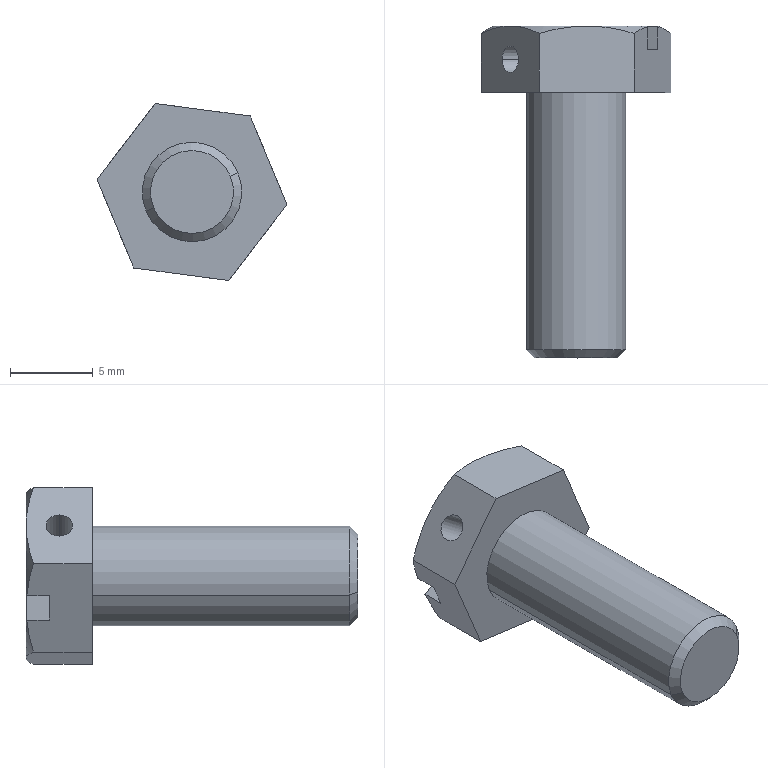Part | SolidWorks | features BaseBody 1 | 1 solid | 26 faces | box 11.449 x 20 x 10.666 mm | volume 753.247 mm3 | plane 14 | cone 8 | cylinder 4 | commonest cylinder face diameters 1.6 x2 6 x2
STEP:
#1=CARTESIAN_POINT('',(325.991,230.1,-29.958));
#2=VERTEX_POINT('',#1);
#3=CARTESIAN_POINT('',(330.609,230.1,-28.042));
#4=VERTEX_POINT('',#3);
#5=CARTESIAN_POINT('',(328.3,230.1,-29.));
#6=DIRECTION('',(0.,-1.,0.));
#7=DIRECTION('',(-0.9237,0.,-0.383));
#8=AXIS2_PLACEMENT_3D('',#5,#6,#7);
#9=CIRCLE('',#8,2.5);
#10=EDGE_CURVE('',#2,#4,#9,.T.);
#11=ORIENTED_EDGE('',*,*,#10,.F.);
#12=CARTESIAN_POINT('',(325.529,230.6,-30.149));
#13=VERTEX_POINT('',#12);
#14=CARTESIAN_POINT('',(325.529,230.6,-30.149));
#15=DIRECTION('',(-0.6532,0.7071,-0.2709));
#16=VECTOR('',#15,1000.);
#17=LINE('',#14,#16);
#18=EDGE_CURVE('',#2,#13,#17,.T.);
#19=ORIENTED_EDGE('',*,*,#18,.T.);
#20=CARTESIAN_POINT('',(331.071,230.6,-27.851));
#21=VERTEX_POINT('',#20);
#22=CARTESIAN_POINT('',(328.3,230.6,-29.));
#23=DIRECTION('',(0.,1.,0.));
#24=DIRECTION('',(-0.9237,0.,-0.383));
#25=AXIS2_PLACEMENT_3D('',#22,#23,#24);
#26=CIRCLE('',#25,3.);
#27=EDGE_CURVE('',#21,#13,#26,.T.);
#28=ORIENTED_EDGE('',*,*,#27,.F.);
#29=CARTESIAN_POINT('',(331.071,230.6,-27.851));
#30=DIRECTION('',(0.6532,0.7071,0.2709));
#31=VECTOR('',#30,1000.);
#32=LINE('',#29,#31);
#33=EDGE_CURVE('',#4,#21,#32,.T.);
#34=ORIENTED_EDGE('',*,*,#33,.F.);
#35=EDGE_LOOP('',(#11,#19,#28,#34));
#36=FACE_OUTER_BOUND('',#35,.T.);
#37=CARTESIAN_POINT('',(328.3,230.6,-29.));
#38=DIRECTION('',(0.,1.,0.));
#39=DIRECTION('',(0.9237,0.,0.383));
#40=AXIS2_PLACEMENT_3D('',#37,#38,#39);
#41=CONICAL_SURFACE('',#40,3.,0.7854);
#42=ADVANCED_FACE('',(#36),#41,.T.);
#43=CARTESIAN_POINT('',(332.755,248.1,-31.407));
#44=VERTEX_POINT('',#43);
#45=CARTESIAN_POINT('',(331.781,248.1,-32.677));
#46=VERTEX_POINT('',#45);
#47=CARTESIAN_POINT('',(332.268,248.1,-32.042));
#48=DIRECTION('',(0.7936,0.,-0.6084));
#49=DIRECTION('',(-0.6084,0.,-0.7936));
#50=AXIS2_PLACEMENT_3D('',#47,#48,#49);
#51=CIRCLE('',#50,0.8);
#52=EDGE_CURVE('',#44,#46,#51,.T.);
#53=ORIENTED_EDGE('',*,*,#52,.T.);
#54=CARTESIAN_POINT('',(323.845,248.1,-26.593));
#55=VERTEX_POINT('',#54);
#56=CARTESIAN_POINT('',(333.766,248.1,-34.199));
#57=DIRECTION('',(-0.7936,0.,0.6084));
#58=VECTOR('',#57,1000.);
#59=LINE('',#56,#58);
#60=EDGE_CURVE('',#46,#55,#59,.T.);
#61=ORIENTED_EDGE('',*,*,#60,.T.);
#62=CARTESIAN_POINT('',(324.819,248.1,-25.323));
#63=VERTEX_POINT('',#62);
#64=CARTESIAN_POINT('',(324.332,248.1,-25.958));
#65=DIRECTION('',(0.7936,0.,-0.6084));
#66=DIRECTION('',(-0.6084,0.,-0.7936));
#67=AXIS2_PLACEMENT_3D('',#64,#65,#66);
#68=CIRCLE('',#67,0.8);
#69=EDGE_CURVE('',#63,#55,#68,.T.);
#70=ORIENTED_EDGE('',*,*,#69,.F.);
#71=CARTESIAN_POINT('',(334.74,248.1,-32.929));
#72=DIRECTION('',(-0.7936,0.,0.6084));
#73=VECTOR('',#72,1000.);
#74=LINE('',#71,#73);
#75=EDGE_CURVE('',#44,#63,#74,.T.);
#76=ORIENTED_EDGE('',*,*,#75,.F.);
#77=EDGE_LOOP('',(#53,#61,#70,#76));
#78=FACE_OUTER_BOUND('',#77,.T.);
#79=CARTESIAN_POINT('',(334.253,248.1,-33.564));
#80=DIRECTION('',(-0.7936,0.,0.6084));
#81=DIRECTION('',(0.6084,0.,0.7936));
#82=AXIS2_PLACEMENT_3D('',#79,#80,#81);
#83=CYLINDRICAL_SURFACE('',#82,0.8);
#84=ADVANCED_FACE('',(#78),#83,.F.);
#85=ORIENTED_EDGE('',*,*,#27,.T.);
#86=CARTESIAN_POINT('',(325.529,246.1,-30.149));
#87=VERTEX_POINT('',#86);
#88=CARTESIAN_POINT('',(325.529,230.1,-30.149));
#89=DIRECTION('',(0.,1.,0.));
#90=VECTOR('',#89,1000.);
#91=LINE('',#88,#90);
#92=EDGE_CURVE('',#13,#87,#91,.T.);
#93=ORIENTED_EDGE('',*,*,#92,.T.);
#94=CARTESIAN_POINT('',(331.071,246.1,-27.851));
#95=VERTEX_POINT('',#94);
#96=CARTESIAN_POINT('',(328.3,246.1,-29.));
#97=DIRECTION('',(0.,1.,0.));
#98=DIRECTION('',(0.9237,0.,0.383));
#99=AXIS2_PLACEMENT_3D('',#96,#97,#98);
#100=CIRCLE('',#99,3.);
#101=EDGE_CURVE('',#95,#87,#100,.T.);
#102=ORIENTED_EDGE('',*,*,#101,.F.);
#103=CARTESIAN_POINT('',(331.071,230.1,-27.851));
#104=DIRECTION('',(0.,1.,0.));
#105=VECTOR('',#104,1000.);
#106=LINE('',#103,#105);
#107=EDGE_CURVE('',#21,#95,#106,.T.);
#108=ORIENTED_EDGE('',*,*,#107,.F.);
#109=EDGE_LOOP('',(#85,#93,#102,#108));
#110=FACE_OUTER_BOUND('',#109,.T.);
#111=CARTESIAN_POINT('',(328.3,230.1,-29.));
#112=DIRECTION('',(0.,1.,0.));
#113=DIRECTION('',(0.9237,0.,0.383));
#114=AXIS2_PLACEMENT_3D('',#111,#112,#113);
#115=CYLINDRICAL_SURFACE('',#114,3.);
#116=ADVANCED_FACE('',(#110),#115,.T.);
#117=CARTESIAN_POINT('',(326.088,246.1,-23.667));
#118=VERTEX_POINT('',#117);
#119=CARTESIAN_POINT('',(322.576,246.1,-28.249));
#120=VERTEX_POINT('',#119);
#121=CARTESIAN_POINT('',(325.913,246.1,-23.896));
#122=DIRECTION('',(-0.6084,0.,-0.7936));
#123=VECTOR('',#122,1000.);
#124=LINE('',#121,#123);
#125=EDGE_CURVE('',#118,#120,#124,.T.);
#126=ORIENTED_EDGE('',*,*,#125,.F.);
#127=CARTESIAN_POINT('',(326.088,249.653,-23.667));
#128=VERTEX_POINT('',#127);
#129=CARTESIAN_POINT('',(326.088,250.1,-23.667));
#130=DIRECTION('',(0.,-1.,0.));
#131=VECTOR('',#130,1000.);
#132=LINE('',#129,#131);
#133=EDGE_CURVE('',#128,#118,#132,.T.);
#134=ORIENTED_EDGE('',*,*,#133,.F.);
#135=CARTESIAN_POINT('',(324.332,250.1,-25.958));
#136=VERTEX_POINT('',#135);
#137=CARTESIAN_POINT('',(324.332,250.1,-25.958));
#138=CARTESIAN_POINT('',(324.481,250.1,-25.763));
#139=CARTESIAN_POINT('',(324.631,250.089,-25.568));
#140=CARTESIAN_POINT('',(324.927,250.049,-25.182));
#141=CARTESIAN_POINT('',(325.074,250.018,-24.99));
#142=CARTESIAN_POINT('',(325.513,249.902,-24.418));
#143=CARTESIAN_POINT('',(325.802,249.789,-24.041));
#144=CARTESIAN_POINT('',(326.088,249.653,-23.667));
#145=B_SPLINE_CURVE_WITH_KNOTS('',3,(#137,#138,#139,#140,#141,#142,#143,#144),.UNSPECIFIED.,.F.,.F.,(4,2,2,4),(0.002921,0.003649,0.004376,0.005831),.UNSPECIFIED.);
#146=EDGE_CURVE('',#136,#128,#145,.T.);
#147=ORIENTED_EDGE('',*,*,#146,.F.);
#148=CARTESIAN_POINT('',(322.576,249.653,-28.249));
#149=VERTEX_POINT('',#148);
#150=CARTESIAN_POINT('',(322.576,249.653,-28.249));
#151=CARTESIAN_POINT('',(323.15,249.926,-27.499));
#152=CARTESIAN_POINT('',(323.734,250.1,-26.738));
#153=CARTESIAN_POINT('',(324.332,250.1,-25.958));
#154=B_SPLINE_CURVE_WITH_KNOTS('',3,(#150,#151,#152,#153),.UNSPECIFIED.,.F.,.F.,(4,4),(0.000000238,0.002921),.UNSPECIFIED.);
#155=EDGE_CURVE('',#149,#136,#154,.T.);
#156=ORIENTED_EDGE('',*,*,#155,.F.);
#157=CARTESIAN_POINT('',(322.576,250.1,-28.249));
#158=DIRECTION('',(0.,-1.,0.));
#159=VECTOR('',#158,1000.);
#160=LINE('',#157,#159);
#161=EDGE_CURVE('',#149,#120,#160,.T.);
#162=ORIENTED_EDGE('',*,*,#161,.T.);
#163=EDGE_LOOP('',(#126,#134,#147,#156,#162));
#164=FACE_OUTER_BOUND('',#163,.T.);
#165=ORIENTED_EDGE('',*,*,#69,.T.);
#166=CARTESIAN_POINT('',(324.332,248.1,-25.958));
#167=DIRECTION('',(0.7936,0.,-0.6084));
#168=DIRECTION('',(-0.6084,0.,-0.7936));
#169=AXIS2_PLACEMENT_3D('',#166,#167,#168);
#170=CIRCLE('',#169,0.8);
#171=EDGE_CURVE('',#55,#63,#170,.T.);
#172=ORIENTED_EDGE('',*,*,#171,.T.);
#173=EDGE_LOOP('',(#165,#172));
#174=FACE_BOUND('',#173,.T.);
#175=CARTESIAN_POINT('',(326.088,250.1,-23.667));
#176=DIRECTION('',(-0.7936,0.,0.6084));
#177=DIRECTION('',(0.6084,0.,0.7936));
#178=AXIS2_PLACEMENT_3D('',#175,#176,#177);
#179=PLANE('',#178);
#180=ADVANCED_FACE('',(#164,#174),#179,.T.);
#181=CARTESIAN_POINT('',(330.512,246.1,-34.333));
#182=VERTEX_POINT('',#181);
#183=CARTESIAN_POINT('',(334.024,246.1,-29.751));
#184=VERTEX_POINT('',#183);
#185=CARTESIAN_POINT('',(333.849,246.1,-29.98));
#186=DIRECTION('',(0.6084,0.,0.7936));
#187=VECTOR('',#186,1000.);
#188=LINE('',#185,#187);
#189=EDGE_CURVE('',#182,#184,#188,.T.);
#190=ORIENTED_EDGE('',*,*,#189,.F.);
#191=CARTESIAN_POINT('',(330.512,249.653,-34.333));
#192=VERTEX_POINT('',#191);
#193=CARTESIAN_POINT('',(330.512,250.1,-34.333));
#194=DIRECTION('',(0.,-1.,0.));
#195=VECTOR('',#194,1000.);
#196=LINE('',#193,#195);
#197=EDGE_CURVE('',#192,#182,#196,.T.);
#198=ORIENTED_EDGE('',*,*,#197,.F.);
#199=CARTESIAN_POINT('',(332.268,250.1,-32.042));
#200=VERTEX_POINT('',#199);
#201=CARTESIAN_POINT('',(332.268,250.1,-32.042));
#202=CARTESIAN_POINT('',(332.119,250.1,-32.237));
#203=CARTESIAN_POINT('',(331.969,250.089,-32.432));
#204=CARTESIAN_POINT('',(331.673,250.049,-32.818));
#205=CARTESIAN_POINT('',(331.526,250.018,-33.01));
#206=CARTESIAN_POINT('',(331.087,249.902,-33.582));
#207=CARTESIAN_POINT('',(330.798,249.789,-33.959));
#208=CARTESIAN_POINT('',(330.512,249.653,-34.333));
#209=B_SPLINE_CURVE_WITH_KNOTS('',3,(#201,#202,#203,#204,#205,#206,#207,#208),.UNSPECIFIED.,.F.,.F.,(4,2,2,4),(0.002921,0.003649,0.004376,0.005831),.UNSPECIFIED.);
#210=EDGE_CURVE('',#200,#192,#209,.T.);
#211=ORIENTED_EDGE('',*,*,#210,.F.);
#212=CARTESIAN_POINT('',(334.024,249.653,-29.751));
#213=VERTEX_POINT('',#212);
#214=CARTESIAN_POINT('',(334.024,249.653,-29.751));
#215=CARTESIAN_POINT('',(333.45,249.926,-30.501));
#216=CARTESIAN_POINT('',(332.866,250.1,-31.262));
#217=CARTESIAN_POINT('',(332.268,250.1,-32.042));
#218=B_SPLINE_CURVE_WITH_KNOTS('',3,(#214,#215,#216,#217),.UNSPECIFIED.,.F.,.F.,(4,4),(0.000000238,0.002921),.UNSPECIFIED.);
#219=EDGE_CURVE('',#213,#200,#218,.T.);
#220=ORIENTED_EDGE('',*,*,#219,.F.);
#221=CARTESIAN_POINT('',(334.024,250.1,-29.751));
#222=DIRECTION('',(0.,-1.,0.));
#223=VECTOR('',#222,1000.);
#224=LINE('',#221,#223);
#225=EDGE_CURVE('',#213,#184,#224,.T.);
#226=ORIENTED_EDGE('',*,*,#225,.T.);
#227=EDGE_LOOP('',(#190,#198,#211,#220,#226));
#228=FACE_OUTER_BOUND('',#227,.T.);
#229=ORIENTED_EDGE('',*,*,#52,.F.);
#230=CARTESIAN_POINT('',(332.268,248.1,-32.042));
#231=DIRECTION('',(0.7936,0.,-0.6084));
#232=DIRECTION('',(-0.6084,0.,-0.7936));
#233=AXIS2_PLACEMENT_3D('',#230,#231,#232);
#234=CIRCLE('',#233,0.8);
#235=EDGE_CURVE('',#46,#44,#234,.T.);
#236=ORIENTED_EDGE('',*,*,#235,.F.);
#237=EDGE_LOOP('',(#229,#236));
#238=FACE_BOUND('',#237,.T.);
#239=CARTESIAN_POINT('',(330.512,250.1,-34.333));
#240=DIRECTION('',(0.7936,0.,-0.6084));
#241=DIRECTION('',(-0.6084,0.,-0.7936));
#242=AXIS2_PLACEMENT_3D('',#239,#240,#241);
#243=PLANE('',#242);
#244=ADVANCED_FACE('',(#228,#238),#243,.T.);
#245=CARTESIAN_POINT('',(328.469,248.7,-29.796));
#246=VERTEX_POINT('',#245);
#247=CARTESIAN_POINT('',(329.597,248.7,-29.328));
#248=VERTEX_POINT('',#247);
#249=CARTESIAN_POINT('',(328.469,248.7,-29.796));
#250=CARTESIAN_POINT('',(328.807,248.98,-29.656));
#251=CARTESIAN_POINT('',(329.259,248.98,-29.468));
#252=CARTESIAN_POINT('',(329.597,248.7,-29.328));
#253=(BOUNDED_CURVE()B_SPLINE_CURVE(3,(#249,#250,#251,#252),.UNSPECIFIED.,.F.,.T.)B_SPLINE_CURVE_WITH_KNOTS((4,4),(0.8481,2.294),.UNSPECIFIED.)CURVE()GEOMETRIC_REPRESENTATION_ITEM()RATIONAL_B_SPLINE_CURVE((1.,0.8333,0.8333,1.))REPRESENTATION_ITEM(''));
#254=EDGE_CURVE('',#246,#248,#253,.T.);
#255=ORIENTED_EDGE('',*,*,#254,.T.);
#256=CARTESIAN_POINT('',(333.225,248.7,-27.824));
#257=VERTEX_POINT('',#256);
#258=CARTESIAN_POINT('',(323.988,248.7,-31.654));
#259=DIRECTION('',(-0.9237,0.,-0.383));
#260=VECTOR('',#259,1000.);
#261=LINE('',#258,#260);
#262=EDGE_CURVE('',#257,#248,#261,.T.);
#263=ORIENTED_EDGE('',*,*,#262,.F.);
#264=CARTESIAN_POINT('',(333.225,250.063,-27.824));
#265=VERTEX_POINT('',#264);
#266=CARTESIAN_POINT('',(333.225,248.7,-27.824));
#267=DIRECTION('',(0.,1.,0.));
#268=VECTOR('',#267,1000.);
#269=LINE('',#266,#268);
#270=EDGE_CURVE('',#257,#265,#269,.T.);
#271=ORIENTED_EDGE('',*,*,#270,.T.);
#272=CARTESIAN_POINT('',(333.166,250.1,-27.848));
#273=VERTEX_POINT('',#272);
#274=CARTESIAN_POINT('',(333.225,250.063,-27.824));
#275=CARTESIAN_POINT('',(333.205,250.076,-27.832));
#276=CARTESIAN_POINT('',(333.185,250.088,-27.84));
#277=CARTESIAN_POINT('',(333.166,250.1,-27.848));
#278=B_SPLINE_CURVE_WITH_KNOTS('',3,(#274,#275,#276,#277),.UNSPECIFIED.,.F.,.F.,(4,4),(0.004516,0.00459),.UNSPECIFIED.);
#279=EDGE_CURVE('',#265,#273,#278,.T.);
#280=ORIENTED_EDGE('',*,*,#279,.T.);
#281=CARTESIAN_POINT('',(324.047,250.1,-31.63));
#282=VERTEX_POINT('',#281);
#283=CARTESIAN_POINT('',(323.988,250.1,-31.654));
#284=DIRECTION('',(-0.9237,0.,-0.383));
#285=VECTOR('',#284,1000.);
#286=LINE('',#283,#285);
#287=EDGE_CURVE('',#273,#282,#286,.T.);
#288=ORIENTED_EDGE('',*,*,#287,.T.);
#289=CARTESIAN_POINT('',(323.988,250.063,-31.654));
#290=VERTEX_POINT('',#289);
#291=CARTESIAN_POINT('',(324.047,250.1,-31.63));
#292=CARTESIAN_POINT('',(324.027,250.088,-31.638));
#293=CARTESIAN_POINT('',(324.008,250.076,-31.646));
#294=CARTESIAN_POINT('',(323.988,250.063,-31.654));
#295=B_SPLINE_CURVE_WITH_KNOTS('',3,(#291,#292,#293,#294),.UNSPECIFIED.,.F.,.F.,(4,4),(0.004802,0.004876),.UNSPECIFIED.);
#296=EDGE_CURVE('',#282,#290,#295,.T.);
#297=ORIENTED_EDGE('',*,*,#296,.T.);
#298=CARTESIAN_POINT('',(323.988,248.7,-31.654));
#299=VERTEX_POINT('',#298);
#300=CARTESIAN_POINT('',(323.988,248.7,-31.654));
#301=DIRECTION('',(0.,1.,0.));
#302=VECTOR('',#301,1000.);
#303=LINE('',#300,#302);
#304=EDGE_CURVE('',#299,#290,#303,.T.);
#305=ORIENTED_EDGE('',*,*,#304,.F.);
#306=CARTESIAN_POINT('',(323.988,248.7,-31.654));
#307=DIRECTION('',(-0.9237,0.,-0.383));
#308=VECTOR('',#307,1000.);
#309=LINE('',#306,#308);
#310=EDGE_CURVE('',#246,#299,#309,.T.);
#311=ORIENTED_EDGE('',*,*,#310,.F.);
#312=EDGE_LOOP('',(#255,#263,#271,#280,#288,#297,#305,#311));
#313=FACE_OUTER_BOUND('',#312,.T.);
#314=CARTESIAN_POINT('',(323.988,248.7,-31.654));
#315=DIRECTION('',(0.383,0.,-0.9237));
#316=DIRECTION('',(-0.9237,0.,-0.383));
#317=AXIS2_PLACEMENT_3D('',#314,#315,#316);
#318=PLANE('',#317);
#319=ADVANCED_FACE('',(#313),#318,.F.);
#320=CARTESIAN_POINT('',(328.131,248.7,-28.204));
#321=VERTEX_POINT('',#320);
#322=CARTESIAN_POINT('',(327.003,248.7,-28.672));
#323=VERTEX_POINT('',#322);
#324=CARTESIAN_POINT('',(328.131,248.7,-28.204));
#325=CARTESIAN_POINT('',(327.793,248.98,-28.344));
#326=CARTESIAN_POINT('',(327.341,248.98,-28.532));
#327=CARTESIAN_POINT('',(327.003,248.7,-28.672));
#328=(BOUNDED_CURVE()B_SPLINE_CURVE(3,(#324,#325,#326,#327),.UNSPECIFIED.,.F.,.T.)B_SPLINE_CURVE_WITH_KNOTS((4,4),(3.99,5.435),.UNSPECIFIED.)CURVE()GEOMETRIC_REPRESENTATION_ITEM()RATIONAL_B_SPLINE_CURVE((1.,0.8333,0.8333,1.))REPRESENTATION_ITEM(''));
#329=EDGE_CURVE('',#321,#323,#328,.T.);
#330=ORIENTED_EDGE('',*,*,#329,.T.);
#331=CARTESIAN_POINT('',(323.375,248.7,-30.176));
#332=VERTEX_POINT('',#331);
#333=CARTESIAN_POINT('',(323.375,248.7,-30.176));
#334=DIRECTION('',(0.9237,0.,0.383));
#335=VECTOR('',#334,1000.);
#336=LINE('',#333,#335);
#337=EDGE_CURVE('',#332,#323,#336,.T.);
#338=ORIENTED_EDGE('',*,*,#337,.F.);
#339=CARTESIAN_POINT('',(323.375,250.063,-30.176));
#340=VERTEX_POINT('',#339);
#341=CARTESIAN_POINT('',(323.375,248.7,-30.176));
#342=DIRECTION('',(0.,1.,0.));
#343=VECTOR('',#342,1000.);
#344=LINE('',#341,#343);
#345=EDGE_CURVE('',#332,#340,#344,.T.);
#346=ORIENTED_EDGE('',*,*,#345,.T.);
#347=CARTESIAN_POINT('',(323.434,250.1,-30.152));
#348=VERTEX_POINT('',#347);
#349=CARTESIAN_POINT('',(323.375,250.063,-30.176));
#350=CARTESIAN_POINT('',(323.395,250.076,-30.168));
#351=CARTESIAN_POINT('',(323.415,250.088,-30.16));
#352=CARTESIAN_POINT('',(323.434,250.1,-30.152));
#353=B_SPLINE_CURVE_WITH_KNOTS('',3,(#349,#350,#351,#352),.UNSPECIFIED.,.F.,.F.,(4,4),(0.004516,0.00459),.UNSPECIFIED.);
#354=EDGE_CURVE('',#340,#348,#353,.T.);
#355=ORIENTED_EDGE('',*,*,#354,.T.);
#356=CARTESIAN_POINT('',(332.553,250.1,-26.37));
#357=VERTEX_POINT('',#356);
#358=CARTESIAN_POINT('',(323.375,250.1,-30.176));
#359=DIRECTION('',(0.9237,0.,0.383));
#360=VECTOR('',#359,1000.);
#361=LINE('',#358,#360);
#362=EDGE_CURVE('',#348,#357,#361,.T.);
#363=ORIENTED_EDGE('',*,*,#362,.T.);
#364=CARTESIAN_POINT('',(332.612,250.063,-26.346));
#365=VERTEX_POINT('',#364);
#366=CARTESIAN_POINT('',(332.553,250.1,-26.37));
#367=CARTESIAN_POINT('',(332.573,250.088,-26.362));
#368=CARTESIAN_POINT('',(332.592,250.076,-26.354));
#369=CARTESIAN_POINT('',(332.612,250.063,-26.346));
#370=B_SPLINE_CURVE_WITH_KNOTS('',3,(#366,#367,#368,#369),.UNSPECIFIED.,.F.,.F.,(4,4),(0.004802,0.004876),.UNSPECIFIED.);
#371=EDGE_CURVE('',#357,#365,#370,.T.);
#372=ORIENTED_EDGE('',*,*,#371,.T.);
#373=CARTESIAN_POINT('',(332.612,248.7,-26.346));
#374=VERTEX_POINT('',#373);
#375=CARTESIAN_POINT('',(332.612,248.7,-26.346));
#376=DIRECTION('',(0.,1.,0.));
#377=VECTOR('',#376,1000.);
#378=LINE('',#375,#377);
#379=EDGE_CURVE('',#374,#365,#378,.T.);
#380=ORIENTED_EDGE('',*,*,#379,.F.);
#381=CARTESIAN_POINT('',(323.375,248.7,-30.176));
#382=DIRECTION('',(0.9237,0.,0.383));
#383=VECTOR('',#382,1000.);
#384=LINE('',#381,#383);
#385=EDGE_CURVE('',#321,#374,#384,.T.);
#386=ORIENTED_EDGE('',*,*,#385,.F.);
#387=EDGE_LOOP('',(#330,#338,#346,#355,#363,#372,#380,#386));
#388=FACE_OUTER_BOUND('',#387,.T.);
#389=CARTESIAN_POINT('',(323.375,248.7,-30.176));
#390=DIRECTION('',(-0.383,0.,0.9237));
#391=DIRECTION('',(0.9237,0.,0.383));
#392=AXIS2_PLACEMENT_3D('',#389,#390,#391);
#393=PLANE('',#392);
#394=ADVANCED_FACE('',(#388),#393,.F.);
#395=ORIENTED_EDGE('',*,*,#337,.T.);
#396=CARTESIAN_POINT('',(333.931,248.7,-33.984));
#397=DIRECTION('',(-0.7936,0.,0.6084));
#398=VECTOR('',#397,1000.);
#399=LINE('',#396,#398);
#400=EDGE_CURVE('',#246,#323,#399,.T.);
#401=ORIENTED_EDGE('',*,*,#400,.F.);
#402=ORIENTED_EDGE('',*,*,#310,.T.);
#403=CARTESIAN_POINT('',(323.988,248.7,-31.654));
#404=DIRECTION('',(-0.3831,0.,0.9237));
#405=VECTOR('',#404,1000.);
#406=LINE('',#403,#405);
#407=EDGE_CURVE('',#299,#332,#406,.T.);
#408=ORIENTED_EDGE('',*,*,#407,.T.);
#409=EDGE_LOOP('',(#395,#401,#402,#408));
#410=FACE_OUTER_BOUND('',#409,.T.);
#411=CARTESIAN_POINT('',(323.375,248.7,-30.176));
#412=DIRECTION('',(0.,1.,0.));
#413=DIRECTION('',(0.9237,0.,0.383));
#414=AXIS2_PLACEMENT_3D('',#411,#412,#413);
#415=PLANE('',#414);
#416=ADVANCED_FACE('',(#410),#415,.T.);
#417=ORIENTED_EDGE('',*,*,#262,.T.);
#418=CARTESIAN_POINT('',(334.575,248.7,-33.144));
#419=DIRECTION('',(0.7936,0.,-0.6084));
#420=VECTOR('',#419,1000.);
#421=LINE('',#418,#420);
#422=EDGE_CURVE('',#321,#248,#421,.T.);
#423=ORIENTED_EDGE('',*,*,#422,.F.);
#424=ORIENTED_EDGE('',*,*,#385,.T.);
#425=CARTESIAN_POINT('',(332.612,248.7,-26.346));
#426=DIRECTION('',(0.383,0.,-0.9237));
#427=VECTOR('',#426,1000.);
#428=LINE('',#425,#427);
#429=EDGE_CURVE('',#374,#257,#428,.T.);
#430=ORIENTED_EDGE('',*,*,#429,.T.);
#431=EDGE_LOOP('',(#417,#423,#424,#430));
#432=FACE_OUTER_BOUND('',#431,.T.);
#433=CARTESIAN_POINT('',(323.375,248.7,-30.176));
#434=DIRECTION('',(0.,1.,0.));
#435=DIRECTION('',(0.9237,0.,0.383));
#436=AXIS2_PLACEMENT_3D('',#433,#434,#435);
#437=PLANE('',#436);
#438=ADVANCED_FACE('',(#432),#437,.T.);
#439=ORIENTED_EDGE('',*,*,#287,.F.);
#440=CARTESIAN_POINT('',(328.3,250.1,-29.));
#441=DIRECTION('',(0.,1.,0.));
#442=DIRECTION('',(0.9237,0.,0.383));
#443=AXIS2_PLACEMENT_3D('',#440,#441,#442);
#444=CIRCLE('',#443,5.);
#445=EDGE_CURVE('',#273,#200,#444,.T.);
#446=ORIENTED_EDGE('',*,*,#445,.T.);
#447=CARTESIAN_POINT('',(327.649,250.1,-33.957));
#448=VERTEX_POINT('',#447);
#449=CARTESIAN_POINT('',(328.3,250.1,-29.));
#450=DIRECTION('',(0.,1.,0.));
#451=DIRECTION('',(0.9237,0.,0.383));
#452=AXIS2_PLACEMENT_3D('',#449,#450,#451);
#453=CIRCLE('',#452,5.);
#454=EDGE_CURVE('',#200,#448,#453,.T.);
#455=ORIENTED_EDGE('',*,*,#454,.T.);
#456=CARTESIAN_POINT('',(328.3,250.1,-29.));
#457=DIRECTION('',(0.,1.,0.));
#458=DIRECTION('',(0.9237,0.,0.383));
#459=AXIS2_PLACEMENT_3D('',#456,#457,#458);
#460=CIRCLE('',#459,5.);
#461=EDGE_CURVE('',#448,#282,#460,.T.);
#462=ORIENTED_EDGE('',*,*,#461,.T.);
#463=EDGE_LOOP('',(#439,#446,#455,#462));
#464=FACE_OUTER_BOUND('',#463,.T.);
#465=CARTESIAN_POINT('',(332.919,250.1,-27.085));
#466=DIRECTION('',(0.,1.,0.));
#467=DIRECTION('',(0.9237,0.,0.383));
#468=AXIS2_PLACEMENT_3D('',#465,#466,#467);
#469=PLANE('',#468);
#470=ADVANCED_FACE('',(#464),#469,.T.);
#471=CARTESIAN_POINT('',(328.3,230.1,-29.));
#472=DIRECTION('',(0.,-1.,0.));
#473=DIRECTION('',(-0.9237,0.,-0.383));
#474=AXIS2_PLACEMENT_3D('',#471,#472,#473);
#475=CIRCLE('',#474,2.5);
#476=EDGE_CURVE('',#4,#2,#475,.T.);
#477=ORIENTED_EDGE('',*,*,#476,.T.);
#478=ORIENTED_EDGE('',*,*,#10,.T.);
#479=EDGE_LOOP('',(#477,#478));
#480=FACE_OUTER_BOUND('',#479,.T.);
#481=CARTESIAN_POINT('',(328.3,230.1,-29.));
#482=DIRECTION('',(0.,-1.,0.));
#483=DIRECTION('',(-0.9237,0.,-0.383));
#484=AXIS2_PLACEMENT_3D('',#481,#482,#483);
#485=PLANE('',#484);
#486=ADVANCED_FACE('',(#480),#485,.T.);
#487=ORIENTED_EDGE('',*,*,#92,.F.);
#488=CARTESIAN_POINT('',(328.3,230.6,-29.));
#489=DIRECTION('',(0.,1.,0.));
#490=DIRECTION('',(-0.9237,0.,-0.383));
#491=AXIS2_PLACEMENT_3D('',#488,#489,#490);
#492=CIRCLE('',#491,3.);
#493=EDGE_CURVE('',#13,#21,#492,.T.);
#494=ORIENTED_EDGE('',*,*,#493,.T.);
#495=ORIENTED_EDGE('',*,*,#107,.T.);
#496=CARTESIAN_POINT('',(328.3,246.1,-29.));
#497=DIRECTION('',(0.,1.,0.));
#498=DIRECTION('',(0.9237,0.,0.383));
#499=AXIS2_PLACEMENT_3D('',#496,#497,#498);
#500=CIRCLE('',#499,3.);
#501=EDGE_CURVE('',#87,#95,#500,.T.);
#502=ORIENTED_EDGE('',*,*,#501,.F.);
#503=EDGE_LOOP('',(#487,#494,#495,#502));
#504=FACE_OUTER_BOUND('',#503,.T.);
#505=CARTESIAN_POINT('',(328.3,230.1,-29.));
#506=DIRECTION('',(0.,1.,0.));
#507=DIRECTION('',(0.9237,0.,0.383));
#508=AXIS2_PLACEMENT_3D('',#505,#506,#507);
#509=CYLINDRICAL_SURFACE('',#508,3.);
#510=ADVANCED_FACE('',(#504),#509,.T.);
#511=ORIENTED_EDGE('',*,*,#101,.T.);
#512=ORIENTED_EDGE('',*,*,#501,.T.);
#513=EDGE_LOOP('',(#511,#512));
#514=FACE_BOUND('',#513,.T.);
#515=ORIENTED_EDGE('',*,*,#125,.T.);
#516=CARTESIAN_POINT('',(324.787,246.1,-33.582));
#517=VERTEX_POINT('',#516);
#518=CARTESIAN_POINT('',(323.681,246.1,-30.915));
#519=DIRECTION('',(0.383,0.,-0.9237));
#520=VECTOR('',#519,1000.);
#521=LINE('',#518,#520);
#522=EDGE_CURVE('',#120,#517,#521,.T.);
#523=ORIENTED_EDGE('',*,*,#522,.T.);
#524=CARTESIAN_POINT('',(330.225,246.1,-34.296));
#525=DIRECTION('',(0.9915,0.,-0.1301));
#526=VECTOR('',#525,1000.);
#527=LINE('',#524,#526);
#528=EDGE_CURVE('',#517,#182,#527,.T.);
#529=ORIENTED_EDGE('',*,*,#528,.T.);
#530=ORIENTED_EDGE('',*,*,#189,.T.);
#531=CARTESIAN_POINT('',(331.813,246.1,-24.418));
#532=VERTEX_POINT('',#531);
#533=CARTESIAN_POINT('',(332.919,246.1,-27.085));
#534=DIRECTION('',(-0.383,0.,0.9237));
#535=VECTOR('',#534,1000.);
#536=LINE('',#533,#535);
#537=EDGE_CURVE('',#184,#532,#536,.T.);
#538=ORIENTED_EDGE('',*,*,#537,.T.);
#539=CARTESIAN_POINT('',(331.527,246.1,-24.381));
#540=DIRECTION('',(-0.9915,0.,0.1301));
#541=VECTOR('',#540,1000.);
#542=LINE('',#539,#541);
#543=EDGE_CURVE('',#532,#118,#542,.T.);
#544=ORIENTED_EDGE('',*,*,#543,.T.);
#545=EDGE_LOOP('',(#515,#523,#529,#530,#538,#544));
#546=FACE_OUTER_BOUND('',#545,.T.);
#547=CARTESIAN_POINT('',(331.071,246.1,-27.851));
#548=DIRECTION('',(0.,-1.,0.));
#549=DIRECTION('',(-0.9237,0.,-0.383));
#550=AXIS2_PLACEMENT_3D('',#547,#548,#549);
#551=PLANE('',#550);
#552=ADVANCED_FACE('',(#514,#546),#551,.T.);
#553=ORIENTED_EDGE('',*,*,#304,.T.);
#554=CARTESIAN_POINT('',(324.787,249.653,-33.582));
#555=VERTEX_POINT('',#554);
#556=CARTESIAN_POINT('',(324.787,249.653,-33.582));
#557=CARTESIAN_POINT('',(324.527,249.85,-32.954));
#558=CARTESIAN_POINT('',(324.262,249.998,-32.315));
#559=CARTESIAN_POINT('',(323.988,250.063,-31.654));
#560=B_SPLINE_CURVE_WITH_KNOTS('',3,(#556,#557,#558,#559),.UNSPECIFIED.,.F.,.F.,(4,4),(0.002116,0.004237),.UNSPECIFIED.);
#561=EDGE_CURVE('',#555,#290,#560,.T.);
#562=ORIENTED_EDGE('',*,*,#561,.F.);
#563=CARTESIAN_POINT('',(324.787,250.1,-33.582));
#564=DIRECTION('',(0.,-1.,0.));
#565=VECTOR('',#564,1000.);
#566=LINE('',#563,#565);
#567=EDGE_CURVE('',#555,#517,#566,.T.);
#568=ORIENTED_EDGE('',*,*,#567,.T.);
#569=ORIENTED_EDGE('',*,*,#522,.F.);
#570=ORIENTED_EDGE('',*,*,#161,.F.);
#571=CARTESIAN_POINT('',(323.375,250.063,-30.176));
#572=CARTESIAN_POINT('',(323.24,250.031,-29.851));
#573=CARTESIAN_POINT('',(323.106,249.979,-29.528));
#574=CARTESIAN_POINT('',(322.839,249.839,-28.884));
#575=CARTESIAN_POINT('',(322.706,249.752,-28.563));
#576=CARTESIAN_POINT('',(322.576,249.653,-28.249));
#577=B_SPLINE_CURVE_WITH_KNOTS('',3,(#571,#572,#573,#574,#575,#576),.UNSPECIFIED.,.F.,.F.,(4,2,4),(0.00583,0.006887,0.007944),.UNSPECIFIED.);
#578=EDGE_CURVE('',#340,#149,#577,.T.);
#579=ORIENTED_EDGE('',*,*,#578,.F.);
#580=ORIENTED_EDGE('',*,*,#345,.F.);
#581=ORIENTED_EDGE('',*,*,#407,.F.);
#582=EDGE_LOOP('',(#553,#562,#568,#569,#570,#579,#580,#581));
#583=FACE_OUTER_BOUND('',#582,.T.);
#584=CARTESIAN_POINT('',(322.576,250.1,-28.249));
#585=DIRECTION('',(-0.9237,0.,-0.383));
#586=DIRECTION('',(-0.383,0.,0.9237));
#587=AXIS2_PLACEMENT_3D('',#584,#585,#586);
#588=PLANE('',#587);
#589=ADVANCED_FACE('',(#583),#588,.T.);
#590=ORIENTED_EDGE('',*,*,#543,.F.);
#591=CARTESIAN_POINT('',(331.813,249.653,-24.418));
#592=VERTEX_POINT('',#591);
#593=CARTESIAN_POINT('',(331.813,250.1,-24.418));
#594=DIRECTION('',(0.,-1.,0.));
#595=VECTOR('',#594,1000.);
#596=LINE('',#593,#595);
#597=EDGE_CURVE('',#592,#532,#596,.T.);
#598=ORIENTED_EDGE('',*,*,#597,.F.);
#599=CARTESIAN_POINT('',(328.951,250.1,-24.043));
#600=VERTEX_POINT('',#599);
#601=CARTESIAN_POINT('',(328.951,250.1,-24.043));
#602=CARTESIAN_POINT('',(329.194,250.1,-24.074));
#603=CARTESIAN_POINT('',(329.438,250.089,-24.106));
#604=CARTESIAN_POINT('',(329.92,250.049,-24.17));
#605=CARTESIAN_POINT('',(330.16,250.018,-24.201));
#606=CARTESIAN_POINT('',(330.875,249.902,-24.295));
#607=CARTESIAN_POINT('',(331.346,249.789,-24.357));
#608=CARTESIAN_POINT('',(331.813,249.653,-24.418));
#609=B_SPLINE_CURVE_WITH_KNOTS('',3,(#601,#602,#603,#604,#605,#606,#607,#608),.UNSPECIFIED.,.F.,.F.,(4,2,2,4),(0.002921,0.003649,0.004376,0.005831),.UNSPECIFIED.);
#610=EDGE_CURVE('',#600,#592,#609,.T.);
#611=ORIENTED_EDGE('',*,*,#610,.F.);
#612=CARTESIAN_POINT('',(326.088,249.653,-23.667));
#613=CARTESIAN_POINT('',(327.025,249.926,-23.79));
#614=CARTESIAN_POINT('',(327.975,250.1,-23.915));
#615=CARTESIAN_POINT('',(328.951,250.1,-24.043));
#616=B_SPLINE_CURVE_WITH_KNOTS('',3,(#612,#613,#614,#615),.UNSPECIFIED.,.F.,.F.,(4,4),(0.000000238,0.002921),.UNSPECIFIED.);
#617=EDGE_CURVE('',#128,#600,#616,.T.);
#618=ORIENTED_EDGE('',*,*,#617,.F.);
#619=ORIENTED_EDGE('',*,*,#133,.T.);
#620=EDGE_LOOP('',(#590,#598,#611,#618,#619));
#621=FACE_OUTER_BOUND('',#620,.T.);
#622=CARTESIAN_POINT('',(331.813,250.1,-24.418));
#623=DIRECTION('',(0.1301,0.,0.9915));
#624=DIRECTION('',(0.9915,0.,-0.1301));
#625=AXIS2_PLACEMENT_3D('',#622,#623,#624);
#626=PLANE('',#625);
#627=ADVANCED_FACE('',(#621),#626,.T.);
#628=ORIENTED_EDGE('',*,*,#270,.F.);
#629=ORIENTED_EDGE('',*,*,#429,.F.);
#630=ORIENTED_EDGE('',*,*,#379,.T.);
#631=CARTESIAN_POINT('',(331.813,249.653,-24.418));
#632=CARTESIAN_POINT('',(331.943,249.752,-24.733));
#633=CARTESIAN_POINT('',(332.076,249.839,-25.053));
#634=CARTESIAN_POINT('',(332.343,249.979,-25.698));
#635=CARTESIAN_POINT('',(332.478,250.031,-26.021));
#636=CARTESIAN_POINT('',(332.612,250.063,-26.346));
#637=B_SPLINE_CURVE_WITH_KNOTS('',3,(#631,#632,#633,#634,#635,#636),.UNSPECIFIED.,.F.,.F.,(4,2,4),(0.00515,0.00621,0.00727),.UNSPECIFIED.);
#638=EDGE_CURVE('',#592,#365,#637,.T.);
#639=ORIENTED_EDGE('',*,*,#638,.F.);
#640=ORIENTED_EDGE('',*,*,#597,.T.);
#641=ORIENTED_EDGE('',*,*,#537,.F.);
#642=ORIENTED_EDGE('',*,*,#225,.F.);
#643=CARTESIAN_POINT('',(333.225,250.063,-27.824));
#644=CARTESIAN_POINT('',(333.499,249.998,-28.484));
#645=CARTESIAN_POINT('',(333.764,249.85,-29.124));
#646=CARTESIAN_POINT('',(334.024,249.653,-29.751));
#647=B_SPLINE_CURVE_WITH_KNOTS('',3,(#643,#644,#645,#646),.UNSPECIFIED.,.F.,.F.,(4,4),(0.008866,0.01099),.UNSPECIFIED.);
#648=EDGE_CURVE('',#265,#213,#647,.T.);
#649=ORIENTED_EDGE('',*,*,#648,.F.);
#650=EDGE_LOOP('',(#628,#629,#630,#639,#640,#641,#642,#649));
#651=FACE_OUTER_BOUND('',#650,.T.);
#652=CARTESIAN_POINT('',(334.024,250.1,-29.751));
#653=DIRECTION('',(0.9237,0.,0.383));
#654=DIRECTION('',(0.383,0.,-0.9237));
#655=AXIS2_PLACEMENT_3D('',#652,#653,#654);
#656=PLANE('',#655);
#657=ADVANCED_FACE('',(#651),#656,.T.);
#658=ORIENTED_EDGE('',*,*,#528,.F.);
#659=ORIENTED_EDGE('',*,*,#567,.F.);
#660=CARTESIAN_POINT('',(327.649,250.1,-33.957));
#661=CARTESIAN_POINT('',(327.406,250.1,-33.926));
#662=CARTESIAN_POINT('',(327.162,250.089,-33.894));
#663=CARTESIAN_POINT('',(326.68,250.049,-33.83));
#664=CARTESIAN_POINT('',(326.44,250.018,-33.799));
#665=CARTESIAN_POINT('',(325.725,249.902,-33.705));
#666=CARTESIAN_POINT('',(325.254,249.789,-33.643));
#667=CARTESIAN_POINT('',(324.787,249.653,-33.582));
#668=B_SPLINE_CURVE_WITH_KNOTS('',3,(#660,#661,#662,#663,#664,#665,#666,#667),.UNSPECIFIED.,.F.,.F.,(4,2,2,4),(0.002921,0.003649,0.004376,0.005831),.UNSPECIFIED.);
#669=EDGE_CURVE('',#448,#555,#668,.T.);
#670=ORIENTED_EDGE('',*,*,#669,.F.);
#671=CARTESIAN_POINT('',(330.512,249.653,-34.333));
#672=CARTESIAN_POINT('',(329.575,249.926,-34.21));
#673=CARTESIAN_POINT('',(328.625,250.1,-34.085));
#674=CARTESIAN_POINT('',(327.649,250.1,-33.957));
#675=B_SPLINE_CURVE_WITH_KNOTS('',3,(#671,#672,#673,#674),.UNSPECIFIED.,.F.,.F.,(4,4),(0.000000238,0.002921),.UNSPECIFIED.);
#676=EDGE_CURVE('',#192,#448,#675,.T.);
#677=ORIENTED_EDGE('',*,*,#676,.F.);
#678=ORIENTED_EDGE('',*,*,#197,.T.);
#679=EDGE_LOOP('',(#658,#659,#670,#677,#678));
#680=FACE_OUTER_BOUND('',#679,.T.);
#681=CARTESIAN_POINT('',(324.787,250.1,-33.582));
#682=DIRECTION('',(-0.1301,0.,-0.9915));
#683=DIRECTION('',(-0.9915,0.,0.1301));
#684=AXIS2_PLACEMENT_3D('',#681,#682,#683);
#685=PLANE('',#684);
#686=ADVANCED_FACE('',(#680),#685,.T.);
#687=ORIENTED_EDGE('',*,*,#371,.F.);
#688=CARTESIAN_POINT('',(328.3,250.1,-29.));
#689=DIRECTION('',(0.,1.,0.));
#690=DIRECTION('',(0.9237,0.,0.383));
#691=AXIS2_PLACEMENT_3D('',#688,#689,#690);
#692=CIRCLE('',#691,5.);
#693=EDGE_CURVE('',#600,#357,#692,.T.);
#694=ORIENTED_EDGE('',*,*,#693,.F.);
#695=ORIENTED_EDGE('',*,*,#610,.T.);
#696=ORIENTED_EDGE('',*,*,#638,.T.);
#697=EDGE_LOOP('',(#687,#694,#695,#696));
#698=FACE_OUTER_BOUND('',#697,.T.);
#699=CARTESIAN_POINT('',(328.3,250.1,-29.));
#700=DIRECTION('',(0.,-1.,0.));
#701=DIRECTION('',(-0.9237,0.,-0.383));
#702=AXIS2_PLACEMENT_3D('',#699,#700,#701);
#703=CONICAL_SURFACE('',#702,5.,1.047);
#704=ADVANCED_FACE('',(#698),#703,.T.);
#705=CARTESIAN_POINT('',(328.3,250.1,-29.));
#706=DIRECTION('',(0.,1.,0.));
#707=DIRECTION('',(0.9237,0.,0.383));
#708=AXIS2_PLACEMENT_3D('',#705,#706,#707);
#709=CIRCLE('',#708,5.);
#710=EDGE_CURVE('',#136,#600,#709,.T.);
#711=ORIENTED_EDGE('',*,*,#710,.F.);
#712=ORIENTED_EDGE('',*,*,#146,.T.);
#713=ORIENTED_EDGE('',*,*,#617,.T.);
#714=EDGE_LOOP('',(#711,#712,#713));
#715=FACE_OUTER_BOUND('',#714,.T.);
#716=CARTESIAN_POINT('',(328.3,250.1,-29.));
#717=DIRECTION('',(0.,-1.,0.));
#718=DIRECTION('',(-0.9237,0.,-0.383));
#719=AXIS2_PLACEMENT_3D('',#716,#717,#718);
#720=CONICAL_SURFACE('',#719,5.,1.047);
#721=ADVANCED_FACE('',(#715),#720,.T.);
#722=ORIENTED_EDGE('',*,*,#354,.F.);
#723=ORIENTED_EDGE('',*,*,#578,.T.);
#724=ORIENTED_EDGE('',*,*,#155,.T.);
#725=CARTESIAN_POINT('',(328.3,250.1,-29.));
#726=DIRECTION('',(0.,1.,0.));
#727=DIRECTION('',(0.9237,0.,0.383));
#728=AXIS2_PLACEMENT_3D('',#725,#726,#727);
#729=CIRCLE('',#728,5.);
#730=EDGE_CURVE('',#348,#136,#729,.T.);
#731=ORIENTED_EDGE('',*,*,#730,.F.);
#732=EDGE_LOOP('',(#722,#723,#724,#731));
#733=FACE_OUTER_BOUND('',#732,.T.);
#734=CARTESIAN_POINT('',(328.3,250.1,-29.));
#735=DIRECTION('',(0.,-1.,0.));
#736=DIRECTION('',(-0.9237,0.,-0.383));
#737=AXIS2_PLACEMENT_3D('',#734,#735,#736);
#738=CONICAL_SURFACE('',#737,5.,1.047);
#739=ADVANCED_FACE('',(#733),#738,.T.);
#740=ORIENTED_EDGE('',*,*,#454,.F.);
#741=ORIENTED_EDGE('',*,*,#210,.T.);
#742=ORIENTED_EDGE('',*,*,#676,.T.);
#743=EDGE_LOOP('',(#740,#741,#742));
#744=FACE_OUTER_BOUND('',#743,.T.);
#745=CARTESIAN_POINT('',(328.3,250.1,-29.));
#746=DIRECTION('',(0.,-1.,0.));
#747=DIRECTION('',(-0.9237,0.,-0.383));
#748=AXIS2_PLACEMENT_3D('',#745,#746,#747);
#749=CONICAL_SURFACE('',#748,5.,1.047);
#750=ADVANCED_FACE('',(#744),#749,.T.);
#751=ORIENTED_EDGE('',*,*,#279,.F.);
#752=ORIENTED_EDGE('',*,*,#648,.T.);
#753=ORIENTED_EDGE('',*,*,#219,.T.);
#754=ORIENTED_EDGE('',*,*,#445,.F.);
#755=EDGE_LOOP('',(#751,#752,#753,#754));
#756=FACE_OUTER_BOUND('',#755,.T.);
#757=CARTESIAN_POINT('',(328.3,250.1,-29.));
#758=DIRECTION('',(0.,-1.,0.));
#759=DIRECTION('',(-0.9237,0.,-0.383));
#760=AXIS2_PLACEMENT_3D('',#757,#758,#759);
#761=CONICAL_SURFACE('',#760,5.,1.047);
#762=ADVANCED_FACE('',(#756),#761,.T.);
#763=ORIENTED_EDGE('',*,*,#362,.F.);
#764=ORIENTED_EDGE('',*,*,#730,.T.);
#765=ORIENTED_EDGE('',*,*,#710,.T.);
#766=ORIENTED_EDGE('',*,*,#693,.T.);
#767=EDGE_LOOP('',(#763,#764,#765,#766));
#768=FACE_OUTER_BOUND('',#767,.T.);
#769=CARTESIAN_POINT('',(332.919,250.1,-27.085));
#770=DIRECTION('',(0.,1.,0.));
#771=DIRECTION('',(0.9237,0.,0.383));
#772=AXIS2_PLACEMENT_3D('',#769,#770,#771);
#773=PLANE('',#772);
#774=ADVANCED_FACE('',(#768),#773,.T.);
#775=ORIENTED_EDGE('',*,*,#296,.F.);
#776=ORIENTED_EDGE('',*,*,#461,.F.);
#777=ORIENTED_EDGE('',*,*,#669,.T.);
#778=ORIENTED_EDGE('',*,*,#561,.T.);
#779=EDGE_LOOP('',(#775,#776,#777,#778));
#780=FACE_OUTER_BOUND('',#779,.T.);
#781=CARTESIAN_POINT('',(328.3,250.1,-29.));
#782=DIRECTION('',(0.,-1.,0.));
#783=DIRECTION('',(-0.9237,0.,-0.383));
#784=AXIS2_PLACEMENT_3D('',#781,#782,#783);
#785=CONICAL_SURFACE('',#784,5.,1.047);
#786=ADVANCED_FACE('',(#780),#785,.T.);
#787=ORIENTED_EDGE('',*,*,#60,.F.);
#788=ORIENTED_EDGE('',*,*,#235,.T.);
#789=ORIENTED_EDGE('',*,*,#75,.T.);
#790=ORIENTED_EDGE('',*,*,#171,.F.);
#791=EDGE_LOOP('',(#787,#788,#789,#790));
#792=FACE_OUTER_BOUND('',#791,.T.);
#793=ORIENTED_EDGE('',*,*,#400,.T.);
#794=ORIENTED_EDGE('',*,*,#329,.F.);
#795=ORIENTED_EDGE('',*,*,#422,.T.);
#796=ORIENTED_EDGE('',*,*,#254,.F.);
#797=EDGE_LOOP('',(#793,#794,#795,#796));
#798=FACE_BOUND('',#797,.T.);
#799=CARTESIAN_POINT('',(334.253,248.1,-33.564));
#800=DIRECTION('',(-0.7936,0.,0.6084));
#801=DIRECTION('',(0.6084,0.,0.7936));
#802=AXIS2_PLACEMENT_3D('',#799,#800,#801);
#803=CYLINDRICAL_SURFACE('',#802,0.8);
#804=ADVANCED_FACE('',(#792,#798),#803,.F.);
#805=ORIENTED_EDGE('',*,*,#18,.F.);
#806=ORIENTED_EDGE('',*,*,#476,.F.);
#807=ORIENTED_EDGE('',*,*,#33,.T.);
#808=ORIENTED_EDGE('',*,*,#493,.F.);
#809=EDGE_LOOP('',(#805,#806,#807,#808));
#810=FACE_OUTER_BOUND('',#809,.T.);
#811=CARTESIAN_POINT('',(328.3,230.6,-29.));
#812=DIRECTION('',(0.,1.,0.));
#813=DIRECTION('',(0.9237,0.,0.383));
#814=AXIS2_PLACEMENT_3D('',#811,#812,#813);
#815=CONICAL_SURFACE('',#814,3.,0.7854);
#816=ADVANCED_FACE('',(#810),#815,.T.);
#817=CLOSED_SHELL('',(#42,#84,#116,#180,#244,#319,#394,#416,#438,#470,#486,#510,#552,#589,#627,#657,#686,#704,#721,#739,#750,#762,#774,#786,#804,#816));
#818=MANIFOLD_SOLID_BREP('',#817);
#819=CARTESIAN_POINT('',(0.,0.,0.));
#820=DIRECTION('',(0.,0.,1.));
#821=DIRECTION('',(1.,0.,0.));
#822=AXIS2_PLACEMENT_3D('',#819,#820,#821);
#823=(LENGTH_UNIT()NAMED_UNIT(*)SI_UNIT(.MILLI.,.METRE.));
#824=UNCERTAINTY_MEASURE_WITH_UNIT(LENGTH_MEASURE(0.00001),#823,'','');
#825=(NAMED_UNIT(*)PLANE_ANGLE_UNIT()SI_UNIT($,.RADIAN.));
#826=(NAMED_UNIT(*)SI_UNIT($,.STERADIAN.)SOLID_ANGLE_UNIT());
#827=(GEOMETRIC_REPRESENTATION_CONTEXT(3)GLOBAL_UNCERTAINTY_ASSIGNED_CONTEXT((#824))GLOBAL_UNIT_ASSIGNED_CONTEXT((#823,#825,#826))REPRESENTATION_CONTEXT('',''));
#828=ADVANCED_BREP_SHAPE_REPRESENTATION('',(#818,#822),#827);